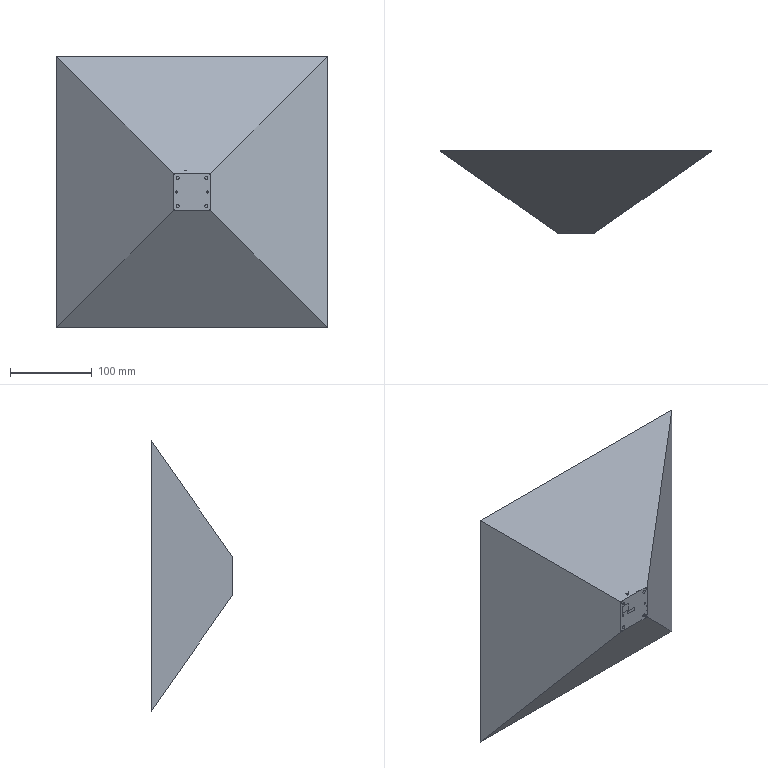Part | SolidWorks | 4 solids | 543 faces | box 331.13 x 100 x 331.13 mm | volume 4244509 mm3 | plane 321 | cylinder 150 | spline 53 | cone 19 | commonest cylinder face diameters 2 x28 3.535 x14 1 x12 1.6 x12 3 x12 5 x12